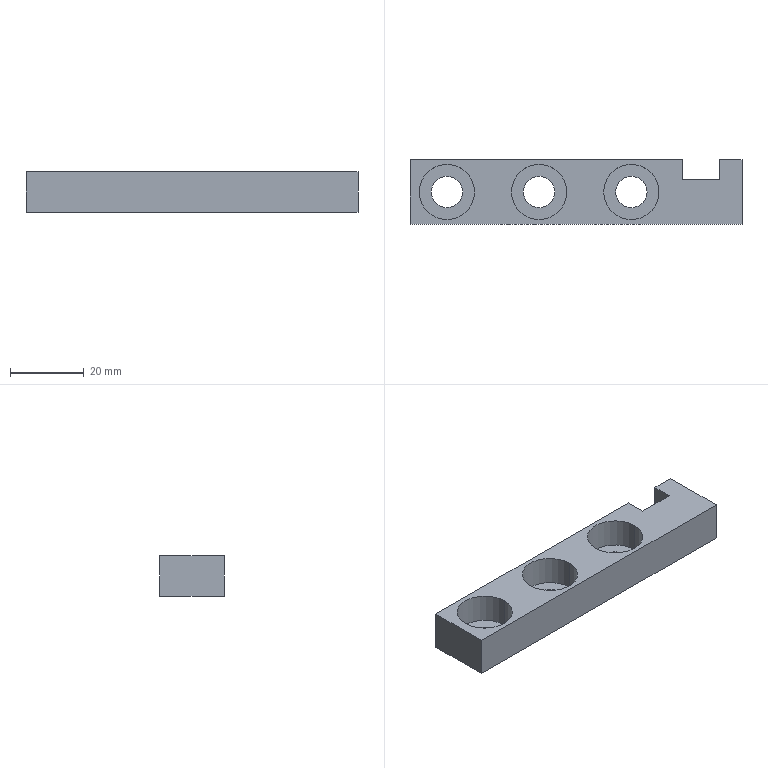Part | SolidWorks | features Extrusion 1, ICE 1 | 1 solid | 25 faces | box 90 x 17.5 x 11 mm | volume 11956 mm3 | plane 13 | cylinder 12 | commonest cylinder face diameters 8.5 x6 15 x6
STEP:
#1=CARTESIAN_POINT('',(-17.5,0.,3.));
#2=VERTEX_POINT('',#1);
#3=CARTESIAN_POINT('',(-2.5,0.,3.));
#4=VERTEX_POINT('',#3);
#5=CARTESIAN_POINT('',(-10.,0.,3.));
#6=DIRECTION('',(0.,0.,1.));
#7=DIRECTION('',(1.,0.,0.));
#8=AXIS2_PLACEMENT_3D('',#5,#6,#7);
#9=CIRCLE('',#8,7.5);
#10=EDGE_CURVE('',#2,#4,#9,.T.);
#11=ORIENTED_EDGE('',*,*,#10,.F.);
#12=CARTESIAN_POINT('',(-17.5,0.,11.));
#13=VERTEX_POINT('',#12);
#14=CARTESIAN_POINT('',(-17.5,0.,3.));
#15=DIRECTION('',(0.,0.,1.));
#16=VECTOR('',#15,1000.);
#17=LINE('',#14,#16);
#18=EDGE_CURVE('',#2,#13,#17,.T.);
#19=ORIENTED_EDGE('',*,*,#18,.T.);
#20=CARTESIAN_POINT('',(-2.5,0.,11.));
#21=VERTEX_POINT('',#20);
#22=CARTESIAN_POINT('',(-10.,0.,11.));
#23=DIRECTION('',(0.,0.,1.));
#24=DIRECTION('',(1.,0.,0.));
#25=AXIS2_PLACEMENT_3D('',#22,#23,#24);
#26=CIRCLE('',#25,7.5);
#27=EDGE_CURVE('',#13,#21,#26,.T.);
#28=ORIENTED_EDGE('',*,*,#27,.T.);
#29=CARTESIAN_POINT('',(-2.5,0.,3.));
#30=DIRECTION('',(0.,0.,1.));
#31=VECTOR('',#30,1000.);
#32=LINE('',#29,#31);
#33=EDGE_CURVE('',#4,#21,#32,.T.);
#34=ORIENTED_EDGE('',*,*,#33,.F.);
#35=EDGE_LOOP('',(#11,#19,#28,#34));
#36=FACE_OUTER_BOUND('',#35,.T.);
#37=CARTESIAN_POINT('',(-10.,0.,3.));
#38=DIRECTION('',(0.,0.,1.));
#39=DIRECTION('',(1.,0.,0.));
#40=AXIS2_PLACEMENT_3D('',#37,#38,#39);
#41=CYLINDRICAL_SURFACE('',#40,7.5);
#42=ADVANCED_FACE('',(#36),#41,.F.);
#43=CARTESIAN_POINT('',(7.5,0.,3.));
#44=VERTEX_POINT('',#43);
#45=CARTESIAN_POINT('',(22.5,0.,3.));
#46=VERTEX_POINT('',#45);
#47=CARTESIAN_POINT('',(15.,0.,3.));
#48=DIRECTION('',(0.,0.,1.));
#49=DIRECTION('',(1.,0.,0.));
#50=AXIS2_PLACEMENT_3D('',#47,#48,#49);
#51=CIRCLE('',#50,7.5);
#52=EDGE_CURVE('',#44,#46,#51,.T.);
#53=ORIENTED_EDGE('',*,*,#52,.F.);
#54=CARTESIAN_POINT('',(7.5,0.,11.));
#55=VERTEX_POINT('',#54);
#56=CARTESIAN_POINT('',(7.5,0.,3.));
#57=DIRECTION('',(0.,0.,1.));
#58=VECTOR('',#57,1000.);
#59=LINE('',#56,#58);
#60=EDGE_CURVE('',#44,#55,#59,.T.);
#61=ORIENTED_EDGE('',*,*,#60,.T.);
#62=CARTESIAN_POINT('',(22.5,0.,11.));
#63=VERTEX_POINT('',#62);
#64=CARTESIAN_POINT('',(15.,0.,11.));
#65=DIRECTION('',(0.,0.,1.));
#66=DIRECTION('',(1.,0.,0.));
#67=AXIS2_PLACEMENT_3D('',#64,#65,#66);
#68=CIRCLE('',#67,7.5);
#69=EDGE_CURVE('',#55,#63,#68,.T.);
#70=ORIENTED_EDGE('',*,*,#69,.T.);
#71=CARTESIAN_POINT('',(22.5,0.,3.));
#72=DIRECTION('',(0.,0.,1.));
#73=VECTOR('',#72,1000.);
#74=LINE('',#71,#73);
#75=EDGE_CURVE('',#46,#63,#74,.T.);
#76=ORIENTED_EDGE('',*,*,#75,.F.);
#77=EDGE_LOOP('',(#53,#61,#70,#76));
#78=FACE_OUTER_BOUND('',#77,.T.);
#79=CARTESIAN_POINT('',(15.,0.,3.));
#80=DIRECTION('',(0.,0.,1.));
#81=DIRECTION('',(1.,0.,0.));
#82=AXIS2_PLACEMENT_3D('',#79,#80,#81);
#83=CYLINDRICAL_SURFACE('',#82,7.5);
#84=ADVANCED_FACE('',(#78),#83,.F.);
#85=CARTESIAN_POINT('',(-42.5,0.,3.));
#86=VERTEX_POINT('',#85);
#87=CARTESIAN_POINT('',(-27.5,0.,3.));
#88=VERTEX_POINT('',#87);
#89=CARTESIAN_POINT('',(-35.,0.,3.));
#90=DIRECTION('',(0.,0.,1.));
#91=DIRECTION('',(1.,0.,0.));
#92=AXIS2_PLACEMENT_3D('',#89,#90,#91);
#93=CIRCLE('',#92,7.5);
#94=EDGE_CURVE('',#86,#88,#93,.T.);
#95=ORIENTED_EDGE('',*,*,#94,.F.);
#96=CARTESIAN_POINT('',(-42.5,0.,11.));
#97=VERTEX_POINT('',#96);
#98=CARTESIAN_POINT('',(-42.5,0.,3.));
#99=DIRECTION('',(0.,0.,1.));
#100=VECTOR('',#99,1000.);
#101=LINE('',#98,#100);
#102=EDGE_CURVE('',#86,#97,#101,.T.);
#103=ORIENTED_EDGE('',*,*,#102,.T.);
#104=CARTESIAN_POINT('',(-27.5,0.,11.));
#105=VERTEX_POINT('',#104);
#106=CARTESIAN_POINT('',(-35.,0.,11.));
#107=DIRECTION('',(0.,0.,1.));
#108=DIRECTION('',(1.,0.,0.));
#109=AXIS2_PLACEMENT_3D('',#106,#107,#108);
#110=CIRCLE('',#109,7.5);
#111=EDGE_CURVE('',#97,#105,#110,.T.);
#112=ORIENTED_EDGE('',*,*,#111,.T.);
#113=CARTESIAN_POINT('',(-27.5,0.,3.));
#114=DIRECTION('',(0.,0.,1.));
#115=VECTOR('',#114,1000.);
#116=LINE('',#113,#115);
#117=EDGE_CURVE('',#88,#105,#116,.T.);
#118=ORIENTED_EDGE('',*,*,#117,.F.);
#119=EDGE_LOOP('',(#95,#103,#112,#118));
#120=FACE_OUTER_BOUND('',#119,.T.);
#121=CARTESIAN_POINT('',(-35.,0.,3.));
#122=DIRECTION('',(0.,0.,1.));
#123=DIRECTION('',(1.,0.,0.));
#124=AXIS2_PLACEMENT_3D('',#121,#122,#123);
#125=CYLINDRICAL_SURFACE('',#124,7.5);
#126=ADVANCED_FACE('',(#120),#125,.F.);
#127=CARTESIAN_POINT('',(-39.25,0.,3.));
#128=VERTEX_POINT('',#127);
#129=CARTESIAN_POINT('',(-30.75,0.,3.));
#130=VERTEX_POINT('',#129);
#131=CARTESIAN_POINT('',(-35.,0.,3.));
#132=DIRECTION('',(0.,0.,1.));
#133=DIRECTION('',(1.,0.,0.));
#134=AXIS2_PLACEMENT_3D('',#131,#132,#133);
#135=CIRCLE('',#134,4.25);
#136=EDGE_CURVE('',#128,#130,#135,.T.);
#137=ORIENTED_EDGE('',*,*,#136,.T.);
#138=CARTESIAN_POINT('',(-30.75,0.,0.));
#139=VERTEX_POINT('',#138);
#140=CARTESIAN_POINT('',(-30.75,0.,11.));
#141=DIRECTION('',(0.,0.,-1.));
#142=VECTOR('',#141,1000.);
#143=LINE('',#140,#142);
#144=EDGE_CURVE('',#130,#139,#143,.T.);
#145=ORIENTED_EDGE('',*,*,#144,.T.);
#146=CARTESIAN_POINT('',(-39.25,0.,0.));
#147=VERTEX_POINT('',#146);
#148=CARTESIAN_POINT('',(-35.,0.,0.));
#149=DIRECTION('',(0.,0.,1.));
#150=DIRECTION('',(1.,0.,0.));
#151=AXIS2_PLACEMENT_3D('',#148,#149,#150);
#152=CIRCLE('',#151,4.25);
#153=EDGE_CURVE('',#147,#139,#152,.T.);
#154=ORIENTED_EDGE('',*,*,#153,.F.);
#155=CARTESIAN_POINT('',(-39.25,0.,11.));
#156=DIRECTION('',(0.,0.,-1.));
#157=VECTOR('',#156,1000.);
#158=LINE('',#155,#157);
#159=EDGE_CURVE('',#128,#147,#158,.T.);
#160=ORIENTED_EDGE('',*,*,#159,.F.);
#161=EDGE_LOOP('',(#137,#145,#154,#160));
#162=FACE_OUTER_BOUND('',#161,.T.);
#163=CARTESIAN_POINT('',(-35.,0.,11.));
#164=DIRECTION('',(0.,0.,-1.));
#165=DIRECTION('',(-1.,0.,0.));
#166=AXIS2_PLACEMENT_3D('',#163,#164,#165);
#167=CYLINDRICAL_SURFACE('',#166,4.25);
#168=ADVANCED_FACE('',(#162),#167,.F.);
#169=CARTESIAN_POINT('',(10.75,0.,3.));
#170=VERTEX_POINT('',#169);
#171=CARTESIAN_POINT('',(19.25,0.,3.));
#172=VERTEX_POINT('',#171);
#173=CARTESIAN_POINT('',(15.,0.,3.));
#174=DIRECTION('',(0.,0.,1.));
#175=DIRECTION('',(1.,0.,0.));
#176=AXIS2_PLACEMENT_3D('',#173,#174,#175);
#177=CIRCLE('',#176,4.25);
#178=EDGE_CURVE('',#170,#172,#177,.T.);
#179=ORIENTED_EDGE('',*,*,#178,.T.);
#180=CARTESIAN_POINT('',(19.25,0.,0.));
#181=VERTEX_POINT('',#180);
#182=CARTESIAN_POINT('',(19.25,0.,11.));
#183=DIRECTION('',(0.,0.,-1.));
#184=VECTOR('',#183,1000.);
#185=LINE('',#182,#184);
#186=EDGE_CURVE('',#172,#181,#185,.T.);
#187=ORIENTED_EDGE('',*,*,#186,.T.);
#188=CARTESIAN_POINT('',(10.75,0.,0.));
#189=VERTEX_POINT('',#188);
#190=CARTESIAN_POINT('',(15.,0.,0.));
#191=DIRECTION('',(0.,0.,1.));
#192=DIRECTION('',(1.,0.,0.));
#193=AXIS2_PLACEMENT_3D('',#190,#191,#192);
#194=CIRCLE('',#193,4.25);
#195=EDGE_CURVE('',#189,#181,#194,.T.);
#196=ORIENTED_EDGE('',*,*,#195,.F.);
#197=CARTESIAN_POINT('',(10.75,0.,11.));
#198=DIRECTION('',(0.,0.,-1.));
#199=VECTOR('',#198,1000.);
#200=LINE('',#197,#199);
#201=EDGE_CURVE('',#170,#189,#200,.T.);
#202=ORIENTED_EDGE('',*,*,#201,.F.);
#203=EDGE_LOOP('',(#179,#187,#196,#202));
#204=FACE_OUTER_BOUND('',#203,.T.);
#205=CARTESIAN_POINT('',(15.,0.,11.));
#206=DIRECTION('',(0.,0.,-1.));
#207=DIRECTION('',(-1.,0.,0.));
#208=AXIS2_PLACEMENT_3D('',#205,#206,#207);
#209=CYLINDRICAL_SURFACE('',#208,4.25);
#210=ADVANCED_FACE('',(#204),#209,.F.);
#211=CARTESIAN_POINT('',(-14.25,0.,3.));
#212=VERTEX_POINT('',#211);
#213=CARTESIAN_POINT('',(-5.75,0.,3.));
#214=VERTEX_POINT('',#213);
#215=CARTESIAN_POINT('',(-10.,0.,3.));
#216=DIRECTION('',(0.,0.,1.));
#217=DIRECTION('',(1.,0.,0.));
#218=AXIS2_PLACEMENT_3D('',#215,#216,#217);
#219=CIRCLE('',#218,4.25);
#220=EDGE_CURVE('',#212,#214,#219,.T.);
#221=ORIENTED_EDGE('',*,*,#220,.T.);
#222=CARTESIAN_POINT('',(-5.75,0.,0.));
#223=VERTEX_POINT('',#222);
#224=CARTESIAN_POINT('',(-5.75,0.,11.));
#225=DIRECTION('',(0.,0.,-1.));
#226=VECTOR('',#225,1000.);
#227=LINE('',#224,#226);
#228=EDGE_CURVE('',#214,#223,#227,.T.);
#229=ORIENTED_EDGE('',*,*,#228,.T.);
#230=CARTESIAN_POINT('',(-14.25,0.,0.));
#231=VERTEX_POINT('',#230);
#232=CARTESIAN_POINT('',(-10.,0.,0.));
#233=DIRECTION('',(0.,0.,1.));
#234=DIRECTION('',(1.,0.,0.));
#235=AXIS2_PLACEMENT_3D('',#232,#233,#234);
#236=CIRCLE('',#235,4.25);
#237=EDGE_CURVE('',#231,#223,#236,.T.);
#238=ORIENTED_EDGE('',*,*,#237,.F.);
#239=CARTESIAN_POINT('',(-14.25,0.,11.));
#240=DIRECTION('',(0.,0.,-1.));
#241=VECTOR('',#240,1000.);
#242=LINE('',#239,#241);
#243=EDGE_CURVE('',#212,#231,#242,.T.);
#244=ORIENTED_EDGE('',*,*,#243,.F.);
#245=EDGE_LOOP('',(#221,#229,#238,#244));
#246=FACE_OUTER_BOUND('',#245,.T.);
#247=CARTESIAN_POINT('',(-10.,0.,11.));
#248=DIRECTION('',(0.,0.,-1.));
#249=DIRECTION('',(-1.,0.,0.));
#250=AXIS2_PLACEMENT_3D('',#247,#248,#249);
#251=CYLINDRICAL_SURFACE('',#250,4.25);
#252=ADVANCED_FACE('',(#246),#251,.F.);
#253=ORIENTED_EDGE('',*,*,#228,.F.);
#254=CARTESIAN_POINT('',(-10.,0.,3.));
#255=DIRECTION('',(0.,0.,1.));
#256=DIRECTION('',(1.,0.,0.));
#257=AXIS2_PLACEMENT_3D('',#254,#255,#256);
#258=CIRCLE('',#257,4.25);
#259=EDGE_CURVE('',#214,#212,#258,.T.);
#260=ORIENTED_EDGE('',*,*,#259,.T.);
#261=ORIENTED_EDGE('',*,*,#243,.T.);
#262=CARTESIAN_POINT('',(-10.,0.,0.));
#263=DIRECTION('',(0.,0.,1.));
#264=DIRECTION('',(1.,0.,0.));
#265=AXIS2_PLACEMENT_3D('',#262,#263,#264);
#266=CIRCLE('',#265,4.25);
#267=EDGE_CURVE('',#223,#231,#266,.T.);
#268=ORIENTED_EDGE('',*,*,#267,.F.);
#269=EDGE_LOOP('',(#253,#260,#261,#268));
#270=FACE_OUTER_BOUND('',#269,.T.);
#271=CARTESIAN_POINT('',(-10.,0.,11.));
#272=DIRECTION('',(0.,0.,-1.));
#273=DIRECTION('',(-1.,0.,0.));
#274=AXIS2_PLACEMENT_3D('',#271,#272,#273);
#275=CYLINDRICAL_SURFACE('',#274,4.25);
#276=ADVANCED_FACE('',(#270),#275,.F.);
#277=ORIENTED_EDGE('',*,*,#186,.F.);
#278=CARTESIAN_POINT('',(15.,0.,3.));
#279=DIRECTION('',(0.,0.,1.));
#280=DIRECTION('',(1.,0.,0.));
#281=AXIS2_PLACEMENT_3D('',#278,#279,#280);
#282=CIRCLE('',#281,4.25);
#283=EDGE_CURVE('',#172,#170,#282,.T.);
#284=ORIENTED_EDGE('',*,*,#283,.T.);
#285=ORIENTED_EDGE('',*,*,#201,.T.);
#286=CARTESIAN_POINT('',(15.,0.,0.));
#287=DIRECTION('',(0.,0.,1.));
#288=DIRECTION('',(1.,0.,0.));
#289=AXIS2_PLACEMENT_3D('',#286,#287,#288);
#290=CIRCLE('',#289,4.25);
#291=EDGE_CURVE('',#181,#189,#290,.T.);
#292=ORIENTED_EDGE('',*,*,#291,.F.);
#293=EDGE_LOOP('',(#277,#284,#285,#292));
#294=FACE_OUTER_BOUND('',#293,.T.);
#295=CARTESIAN_POINT('',(15.,0.,11.));
#296=DIRECTION('',(0.,0.,-1.));
#297=DIRECTION('',(-1.,0.,0.));
#298=AXIS2_PLACEMENT_3D('',#295,#296,#297);
#299=CYLINDRICAL_SURFACE('',#298,4.25);
#300=ADVANCED_FACE('',(#294),#299,.F.);
#301=ORIENTED_EDGE('',*,*,#144,.F.);
#302=CARTESIAN_POINT('',(-35.,0.,3.));
#303=DIRECTION('',(0.,0.,1.));
#304=DIRECTION('',(1.,0.,0.));
#305=AXIS2_PLACEMENT_3D('',#302,#303,#304);
#306=CIRCLE('',#305,4.25);
#307=EDGE_CURVE('',#130,#128,#306,.T.);
#308=ORIENTED_EDGE('',*,*,#307,.T.);
#309=ORIENTED_EDGE('',*,*,#159,.T.);
#310=CARTESIAN_POINT('',(-35.,0.,0.));
#311=DIRECTION('',(0.,0.,1.));
#312=DIRECTION('',(1.,0.,0.));
#313=AXIS2_PLACEMENT_3D('',#310,#311,#312);
#314=CIRCLE('',#313,4.25);
#315=EDGE_CURVE('',#139,#147,#314,.T.);
#316=ORIENTED_EDGE('',*,*,#315,.F.);
#317=EDGE_LOOP('',(#301,#308,#309,#316));
#318=FACE_OUTER_BOUND('',#317,.T.);
#319=CARTESIAN_POINT('',(-35.,0.,11.));
#320=DIRECTION('',(0.,0.,-1.));
#321=DIRECTION('',(-1.,0.,0.));
#322=AXIS2_PLACEMENT_3D('',#319,#320,#321);
#323=CYLINDRICAL_SURFACE('',#322,4.25);
#324=ADVANCED_FACE('',(#318),#323,.F.);
#325=CARTESIAN_POINT('',(-10.,0.,11.));
#326=DIRECTION('',(0.,0.,1.));
#327=DIRECTION('',(1.,0.,0.));
#328=AXIS2_PLACEMENT_3D('',#325,#326,#327);
#329=CIRCLE('',#328,7.5);
#330=EDGE_CURVE('',#21,#13,#329,.T.);
#331=ORIENTED_EDGE('',*,*,#330,.F.);
#332=ORIENTED_EDGE('',*,*,#27,.F.);
#333=EDGE_LOOP('',(#331,#332));
#334=FACE_BOUND('',#333,.T.);
#335=CARTESIAN_POINT('',(15.,0.,11.));
#336=DIRECTION('',(0.,0.,1.));
#337=DIRECTION('',(1.,0.,0.));
#338=AXIS2_PLACEMENT_3D('',#335,#336,#337);
#339=CIRCLE('',#338,7.5);
#340=EDGE_CURVE('',#63,#55,#339,.T.);
#341=ORIENTED_EDGE('',*,*,#340,.F.);
#342=ORIENTED_EDGE('',*,*,#69,.F.);
#343=EDGE_LOOP('',(#341,#342));
#344=FACE_BOUND('',#343,.T.);
#345=CARTESIAN_POINT('',(-35.,0.,11.));
#346=DIRECTION('',(0.,0.,1.));
#347=DIRECTION('',(1.,0.,0.));
#348=AXIS2_PLACEMENT_3D('',#345,#346,#347);
#349=CIRCLE('',#348,7.5);
#350=EDGE_CURVE('',#105,#97,#349,.T.);
#351=ORIENTED_EDGE('',*,*,#350,.F.);
#352=ORIENTED_EDGE('',*,*,#111,.F.);
#353=EDGE_LOOP('',(#351,#352));
#354=FACE_BOUND('',#353,.T.);
#355=CARTESIAN_POINT('',(45.,-8.75,11.));
#356=VERTEX_POINT('',#355);
#357=CARTESIAN_POINT('',(45.,8.75,11.));
#358=VERTEX_POINT('',#357);
#359=CARTESIAN_POINT('',(45.,8.75,11.));
#360=DIRECTION('',(0.,1.,0.));
#361=VECTOR('',#360,1000.);
#362=LINE('',#359,#361);
#363=EDGE_CURVE('',#356,#358,#362,.T.);
#364=ORIENTED_EDGE('',*,*,#363,.T.);
#365=CARTESIAN_POINT('',(39.,8.75,11.));
#366=VERTEX_POINT('',#365);
#367=CARTESIAN_POINT('',(39.,8.75,11.));
#368=DIRECTION('',(-1.,0.,0.));
#369=VECTOR('',#368,1000.);
#370=LINE('',#367,#369);
#371=EDGE_CURVE('',#358,#366,#370,.T.);
#372=ORIENTED_EDGE('',*,*,#371,.T.);
#373=CARTESIAN_POINT('',(39.,3.25,11.));
#374=VERTEX_POINT('',#373);
#375=CARTESIAN_POINT('',(39.,3.25,11.));
#376=DIRECTION('',(0.,-1.,0.));
#377=VECTOR('',#376,1000.);
#378=LINE('',#375,#377);
#379=EDGE_CURVE('',#366,#374,#378,.T.);
#380=ORIENTED_EDGE('',*,*,#379,.T.);
#381=CARTESIAN_POINT('',(28.8,3.25,11.));
#382=VERTEX_POINT('',#381);
#383=CARTESIAN_POINT('',(28.8,3.25,11.));
#384=DIRECTION('',(-1.,0.,0.));
#385=VECTOR('',#384,1000.);
#386=LINE('',#383,#385);
#387=EDGE_CURVE('',#374,#382,#386,.T.);
#388=ORIENTED_EDGE('',*,*,#387,.T.);
#389=CARTESIAN_POINT('',(28.8,8.75,11.));
#390=VERTEX_POINT('',#389);
#391=CARTESIAN_POINT('',(28.8,8.75,11.));
#392=DIRECTION('',(0.,1.,0.));
#393=VECTOR('',#392,1000.);
#394=LINE('',#391,#393);
#395=EDGE_CURVE('',#382,#390,#394,.T.);
#396=ORIENTED_EDGE('',*,*,#395,.T.);
#397=CARTESIAN_POINT('',(-45.,8.75,11.));
#398=VERTEX_POINT('',#397);
#399=CARTESIAN_POINT('',(-45.,8.75,11.));
#400=DIRECTION('',(-1.,0.,0.));
#401=VECTOR('',#400,1000.);
#402=LINE('',#399,#401);
#403=EDGE_CURVE('',#390,#398,#402,.T.);
#404=ORIENTED_EDGE('',*,*,#403,.T.);
#405=CARTESIAN_POINT('',(-45.,-8.75,11.));
#406=VERTEX_POINT('',#405);
#407=CARTESIAN_POINT('',(-45.,8.75,11.));
#408=DIRECTION('',(0.,-1.,0.));
#409=VECTOR('',#408,1000.);
#410=LINE('',#407,#409);
#411=EDGE_CURVE('',#398,#406,#410,.T.);
#412=ORIENTED_EDGE('',*,*,#411,.T.);
#413=CARTESIAN_POINT('',(-45.,-8.75,11.));
#414=DIRECTION('',(1.,0.,0.));
#415=VECTOR('',#414,1000.);
#416=LINE('',#413,#415);
#417=EDGE_CURVE('',#406,#356,#416,.T.);
#418=ORIENTED_EDGE('',*,*,#417,.T.);
#419=EDGE_LOOP('',(#364,#372,#380,#388,#396,#404,#412,#418));
#420=FACE_OUTER_BOUND('',#419,.T.);
#421=CARTESIAN_POINT('',(0.,0.,11.));
#422=DIRECTION('',(0.,0.,1.));
#423=DIRECTION('',(1.,0.,0.));
#424=AXIS2_PLACEMENT_3D('',#421,#422,#423);
#425=PLANE('',#424);
#426=ADVANCED_FACE('',(#334,#344,#354,#420),#425,.T.);
#427=CARTESIAN_POINT('',(45.,-8.75,0.));
#428=VERTEX_POINT('',#427);
#429=CARTESIAN_POINT('',(45.,8.75,0.));
#430=VERTEX_POINT('',#429);
#431=CARTESIAN_POINT('',(45.,8.75,0.));
#432=DIRECTION('',(0.,1.,0.));
#433=VECTOR('',#432,1000.);
#434=LINE('',#431,#433);
#435=EDGE_CURVE('',#428,#430,#434,.T.);
#436=ORIENTED_EDGE('',*,*,#435,.F.);
#437=CARTESIAN_POINT('',(-45.,-8.75,0.));
#438=VERTEX_POINT('',#437);
#439=CARTESIAN_POINT('',(-45.,-8.75,0.));
#440=DIRECTION('',(1.,0.,0.));
#441=VECTOR('',#440,1000.);
#442=LINE('',#439,#441);
#443=EDGE_CURVE('',#438,#428,#442,.T.);
#444=ORIENTED_EDGE('',*,*,#443,.F.);
#445=CARTESIAN_POINT('',(-45.,8.75,0.));
#446=VERTEX_POINT('',#445);
#447=CARTESIAN_POINT('',(-45.,8.75,0.));
#448=DIRECTION('',(0.,-1.,0.));
#449=VECTOR('',#448,1000.);
#450=LINE('',#447,#449);
#451=EDGE_CURVE('',#446,#438,#450,.T.);
#452=ORIENTED_EDGE('',*,*,#451,.F.);
#453=CARTESIAN_POINT('',(28.8,8.75,0.));
#454=VERTEX_POINT('',#453);
#455=CARTESIAN_POINT('',(-45.,8.75,0.));
#456=DIRECTION('',(-1.,0.,0.));
#457=VECTOR('',#456,1000.);
#458=LINE('',#455,#457);
#459=EDGE_CURVE('',#454,#446,#458,.T.);
#460=ORIENTED_EDGE('',*,*,#459,.F.);
#461=CARTESIAN_POINT('',(28.8,3.25,0.));
#462=VERTEX_POINT('',#461);
#463=CARTESIAN_POINT('',(28.8,8.75,0.));
#464=DIRECTION('',(0.,1.,0.));
#465=VECTOR('',#464,1000.);
#466=LINE('',#463,#465);
#467=EDGE_CURVE('',#462,#454,#466,.T.);
#468=ORIENTED_EDGE('',*,*,#467,.F.);
#469=CARTESIAN_POINT('',(39.,3.25,0.));
#470=VERTEX_POINT('',#469);
#471=CARTESIAN_POINT('',(28.8,3.25,0.));
#472=DIRECTION('',(-1.,0.,0.));
#473=VECTOR('',#472,1000.);
#474=LINE('',#471,#473);
#475=EDGE_CURVE('',#470,#462,#474,.T.);
#476=ORIENTED_EDGE('',*,*,#475,.F.);
#477=CARTESIAN_POINT('',(39.,8.75,0.));
#478=VERTEX_POINT('',#477);
#479=CARTESIAN_POINT('',(39.,3.25,0.));
#480=DIRECTION('',(0.,-1.,0.));
#481=VECTOR('',#480,1000.);
#482=LINE('',#479,#481);
#483=EDGE_CURVE('',#478,#470,#482,.T.);
#484=ORIENTED_EDGE('',*,*,#483,.F.);
#485=CARTESIAN_POINT('',(39.,8.75,0.));
#486=DIRECTION('',(-1.,0.,0.));
#487=VECTOR('',#486,1000.);
#488=LINE('',#485,#487);
#489=EDGE_CURVE('',#430,#478,#488,.T.);
#490=ORIENTED_EDGE('',*,*,#489,.F.);
#491=EDGE_LOOP('',(#436,#444,#452,#460,#468,#476,#484,#490));
#492=FACE_OUTER_BOUND('',#491,.T.);
#493=ORIENTED_EDGE('',*,*,#153,.T.);
#494=ORIENTED_EDGE('',*,*,#315,.T.);
#495=EDGE_LOOP('',(#493,#494));
#496=FACE_BOUND('',#495,.T.);
#497=ORIENTED_EDGE('',*,*,#237,.T.);
#498=ORIENTED_EDGE('',*,*,#267,.T.);
#499=EDGE_LOOP('',(#497,#498));
#500=FACE_BOUND('',#499,.T.);
#501=ORIENTED_EDGE('',*,*,#195,.T.);
#502=ORIENTED_EDGE('',*,*,#291,.T.);
#503=EDGE_LOOP('',(#501,#502));
#504=FACE_BOUND('',#503,.T.);
#505=CARTESIAN_POINT('',(0.,0.,0.));
#506=DIRECTION('',(0.,0.,1.));
#507=DIRECTION('',(1.,0.,0.));
#508=AXIS2_PLACEMENT_3D('',#505,#506,#507);
#509=PLANE('',#508);
#510=ADVANCED_FACE('',(#492,#496,#500,#504),#509,.F.);
#511=ORIENTED_EDGE('',*,*,#435,.T.);
#512=CARTESIAN_POINT('',(45.,8.75,11.));
#513=DIRECTION('',(0.,0.,-1.));
#514=VECTOR('',#513,1000.);
#515=LINE('',#512,#514);
#516=EDGE_CURVE('',#358,#430,#515,.T.);
#517=ORIENTED_EDGE('',*,*,#516,.F.);
#518=ORIENTED_EDGE('',*,*,#363,.F.);
#519=CARTESIAN_POINT('',(45.,-8.75,11.));
#520=DIRECTION('',(0.,0.,-1.));
#521=VECTOR('',#520,1000.);
#522=LINE('',#519,#521);
#523=EDGE_CURVE('',#356,#428,#522,.T.);
#524=ORIENTED_EDGE('',*,*,#523,.T.);
#525=EDGE_LOOP('',(#511,#517,#518,#524));
#526=FACE_OUTER_BOUND('',#525,.T.);
#527=CARTESIAN_POINT('',(45.,8.75,11.));
#528=DIRECTION('',(-1.,0.,0.));
#529=DIRECTION('',(0.,0.,1.));
#530=AXIS2_PLACEMENT_3D('',#527,#528,#529);
#531=PLANE('',#530);
#532=ADVANCED_FACE('',(#526),#531,.F.);
#533=ORIENTED_EDGE('',*,*,#489,.T.);
#534=CARTESIAN_POINT('',(39.,8.75,11.));
#535=DIRECTION('',(0.,0.,-1.));
#536=VECTOR('',#535,1000.);
#537=LINE('',#534,#536);
#538=EDGE_CURVE('',#366,#478,#537,.T.);
#539=ORIENTED_EDGE('',*,*,#538,.F.);
#540=ORIENTED_EDGE('',*,*,#371,.F.);
#541=ORIENTED_EDGE('',*,*,#516,.T.);
#542=EDGE_LOOP('',(#533,#539,#540,#541));
#543=FACE_OUTER_BOUND('',#542,.T.);
#544=CARTESIAN_POINT('',(39.,8.75,11.));
#545=DIRECTION('',(0.,-1.,0.));
#546=DIRECTION('',(1.,0.,0.));
#547=AXIS2_PLACEMENT_3D('',#544,#545,#546);
#548=PLANE('',#547);
#549=ADVANCED_FACE('',(#543),#548,.F.);
#550=ORIENTED_EDGE('',*,*,#483,.T.);
#551=CARTESIAN_POINT('',(39.,3.25,11.));
#552=DIRECTION('',(0.,0.,-1.));
#553=VECTOR('',#552,1000.);
#554=LINE('',#551,#553);
#555=EDGE_CURVE('',#374,#470,#554,.T.);
#556=ORIENTED_EDGE('',*,*,#555,.F.);
#557=ORIENTED_EDGE('',*,*,#379,.F.);
#558=ORIENTED_EDGE('',*,*,#538,.T.);
#559=EDGE_LOOP('',(#550,#556,#557,#558));
#560=FACE_OUTER_BOUND('',#559,.T.);
#561=CARTESIAN_POINT('',(39.,3.25,11.));
#562=DIRECTION('',(1.,0.,0.));
#563=DIRECTION('',(0.,0.,-1.));
#564=AXIS2_PLACEMENT_3D('',#561,#562,#563);
#565=PLANE('',#564);
#566=ADVANCED_FACE('',(#560),#565,.F.);
#567=ORIENTED_EDGE('',*,*,#475,.T.);
#568=CARTESIAN_POINT('',(28.8,3.25,11.));
#569=DIRECTION('',(0.,0.,-1.));
#570=VECTOR('',#569,1000.);
#571=LINE('',#568,#570);
#572=EDGE_CURVE('',#382,#462,#571,.T.);
#573=ORIENTED_EDGE('',*,*,#572,.F.);
#574=ORIENTED_EDGE('',*,*,#387,.F.);
#575=ORIENTED_EDGE('',*,*,#555,.T.);
#576=EDGE_LOOP('',(#567,#573,#574,#575));
#577=FACE_OUTER_BOUND('',#576,.T.);
#578=CARTESIAN_POINT('',(28.8,3.25,11.));
#579=DIRECTION('',(0.,-1.,0.));
#580=DIRECTION('',(0.,0.,-1.));
#581=AXIS2_PLACEMENT_3D('',#578,#579,#580);
#582=PLANE('',#581);
#583=ADVANCED_FACE('',(#577),#582,.F.);
#584=ORIENTED_EDGE('',*,*,#467,.T.);
#585=CARTESIAN_POINT('',(28.8,8.75,11.));
#586=DIRECTION('',(0.,0.,-1.));
#587=VECTOR('',#586,1000.);
#588=LINE('',#585,#587);
#589=EDGE_CURVE('',#390,#454,#588,.T.);
#590=ORIENTED_EDGE('',*,*,#589,.F.);
#591=ORIENTED_EDGE('',*,*,#395,.F.);
#592=ORIENTED_EDGE('',*,*,#572,.T.);
#593=EDGE_LOOP('',(#584,#590,#591,#592));
#594=FACE_OUTER_BOUND('',#593,.T.);
#595=CARTESIAN_POINT('',(28.8,8.75,11.));
#596=DIRECTION('',(-1.,0.,0.));
#597=DIRECTION('',(0.,0.,1.));
#598=AXIS2_PLACEMENT_3D('',#595,#596,#597);
#599=PLANE('',#598);
#600=ADVANCED_FACE('',(#594),#599,.F.);
#601=ORIENTED_EDGE('',*,*,#459,.T.);
#602=CARTESIAN_POINT('',(-45.,8.75,11.));
#603=DIRECTION('',(0.,0.,-1.));
#604=VECTOR('',#603,1000.);
#605=LINE('',#602,#604);
#606=EDGE_CURVE('',#398,#446,#605,.T.);
#607=ORIENTED_EDGE('',*,*,#606,.F.);
#608=ORIENTED_EDGE('',*,*,#403,.F.);
#609=ORIENTED_EDGE('',*,*,#589,.T.);
#610=EDGE_LOOP('',(#601,#607,#608,#609));
#611=FACE_OUTER_BOUND('',#610,.T.);
#612=CARTESIAN_POINT('',(-45.,8.75,11.));
#613=DIRECTION('',(0.,-1.,0.));
#614=DIRECTION('',(1.,0.,0.));
#615=AXIS2_PLACEMENT_3D('',#612,#613,#614);
#616=PLANE('',#615);
#617=ADVANCED_FACE('',(#611),#616,.F.);
#618=ORIENTED_EDGE('',*,*,#451,.T.);
#619=CARTESIAN_POINT('',(-45.,-8.75,11.));
#620=DIRECTION('',(0.,0.,-1.));
#621=VECTOR('',#620,1000.);
#622=LINE('',#619,#621);
#623=EDGE_CURVE('',#406,#438,#622,.T.);
#624=ORIENTED_EDGE('',*,*,#623,.F.);
#625=ORIENTED_EDGE('',*,*,#411,.F.);
#626=ORIENTED_EDGE('',*,*,#606,.T.);
#627=EDGE_LOOP('',(#618,#624,#625,#626));
#628=FACE_OUTER_BOUND('',#627,.T.);
#629=CARTESIAN_POINT('',(-45.,8.75,11.));
#630=DIRECTION('',(1.,0.,0.));
#631=DIRECTION('',(0.,0.,-1.));
#632=AXIS2_PLACEMENT_3D('',#629,#630,#631);
#633=PLANE('',#632);
#634=ADVANCED_FACE('',(#628),#633,.F.);
#635=ORIENTED_EDGE('',*,*,#443,.T.);
#636=ORIENTED_EDGE('',*,*,#523,.F.);
#637=ORIENTED_EDGE('',*,*,#417,.F.);
#638=ORIENTED_EDGE('',*,*,#623,.T.);
#639=EDGE_LOOP('',(#635,#636,#637,#638));
#640=FACE_OUTER_BOUND('',#639,.T.);
#641=CARTESIAN_POINT('',(-45.,-8.75,11.));
#642=DIRECTION('',(0.,1.,0.));
#643=DIRECTION('',(0.,0.,1.));
#644=AXIS2_PLACEMENT_3D('',#641,#642,#643);
#645=PLANE('',#644);
#646=ADVANCED_FACE('',(#640),#645,.F.);
#647=ORIENTED_EDGE('',*,*,#102,.F.);
#648=CARTESIAN_POINT('',(-35.,0.,3.));
#649=DIRECTION('',(0.,0.,1.));
#650=DIRECTION('',(1.,0.,0.));
#651=AXIS2_PLACEMENT_3D('',#648,#649,#650);
#652=CIRCLE('',#651,7.5);
#653=EDGE_CURVE('',#88,#86,#652,.T.);
#654=ORIENTED_EDGE('',*,*,#653,.F.);
#655=ORIENTED_EDGE('',*,*,#117,.T.);
#656=ORIENTED_EDGE('',*,*,#350,.T.);
#657=EDGE_LOOP('',(#647,#654,#655,#656));
#658=FACE_OUTER_BOUND('',#657,.T.);
#659=CARTESIAN_POINT('',(-35.,0.,3.));
#660=DIRECTION('',(0.,0.,1.));
#661=DIRECTION('',(1.,0.,0.));
#662=AXIS2_PLACEMENT_3D('',#659,#660,#661);
#663=CYLINDRICAL_SURFACE('',#662,7.5);
#664=ADVANCED_FACE('',(#658),#663,.F.);
#665=ORIENTED_EDGE('',*,*,#136,.F.);
#666=ORIENTED_EDGE('',*,*,#307,.F.);
#667=EDGE_LOOP('',(#665,#666));
#668=FACE_BOUND('',#667,.T.);
#669=ORIENTED_EDGE('',*,*,#653,.T.);
#670=ORIENTED_EDGE('',*,*,#94,.T.);
#671=EDGE_LOOP('',(#669,#670));
#672=FACE_OUTER_BOUND('',#671,.T.);
#673=CARTESIAN_POINT('',(-35.,0.,3.));
#674=DIRECTION('',(0.,0.,1.));
#675=DIRECTION('',(1.,0.,0.));
#676=AXIS2_PLACEMENT_3D('',#673,#674,#675);
#677=PLANE('',#676);
#678=ADVANCED_FACE('',(#668,#672),#677,.T.);
#679=ORIENTED_EDGE('',*,*,#60,.F.);
#680=CARTESIAN_POINT('',(15.,0.,3.));
#681=DIRECTION('',(0.,0.,1.));
#682=DIRECTION('',(1.,0.,0.));
#683=AXIS2_PLACEMENT_3D('',#680,#681,#682);
#684=CIRCLE('',#683,7.5);
#685=EDGE_CURVE('',#46,#44,#684,.T.);
#686=ORIENTED_EDGE('',*,*,#685,.F.);
#687=ORIENTED_EDGE('',*,*,#75,.T.);
#688=ORIENTED_EDGE('',*,*,#340,.T.);
#689=EDGE_LOOP('',(#679,#686,#687,#688));
#690=FACE_OUTER_BOUND('',#689,.T.);
#691=CARTESIAN_POINT('',(15.,0.,3.));
#692=DIRECTION('',(0.,0.,1.));
#693=DIRECTION('',(1.,0.,0.));
#694=AXIS2_PLACEMENT_3D('',#691,#692,#693);
#695=CYLINDRICAL_SURFACE('',#694,7.5);
#696=ADVANCED_FACE('',(#690),#695,.F.);
#697=ORIENTED_EDGE('',*,*,#178,.F.);
#698=ORIENTED_EDGE('',*,*,#283,.F.);
#699=EDGE_LOOP('',(#697,#698));
#700=FACE_BOUND('',#699,.T.);
#701=ORIENTED_EDGE('',*,*,#685,.T.);
#702=ORIENTED_EDGE('',*,*,#52,.T.);
#703=EDGE_LOOP('',(#701,#702));
#704=FACE_OUTER_BOUND('',#703,.T.);
#705=CARTESIAN_POINT('',(15.,0.,3.));
#706=DIRECTION('',(0.,0.,1.));
#707=DIRECTION('',(1.,0.,0.));
#708=AXIS2_PLACEMENT_3D('',#705,#706,#707);
#709=PLANE('',#708);
#710=ADVANCED_FACE('',(#700,#704),#709,.T.);
#711=ORIENTED_EDGE('',*,*,#18,.F.);
#712=CARTESIAN_POINT('',(-10.,0.,3.));
#713=DIRECTION('',(0.,0.,1.));
#714=DIRECTION('',(1.,0.,0.));
#715=AXIS2_PLACEMENT_3D('',#712,#713,#714);
#716=CIRCLE('',#715,7.5);
#717=EDGE_CURVE('',#4,#2,#716,.T.);
#718=ORIENTED_EDGE('',*,*,#717,.F.);
#719=ORIENTED_EDGE('',*,*,#33,.T.);
#720=ORIENTED_EDGE('',*,*,#330,.T.);
#721=EDGE_LOOP('',(#711,#718,#719,#720));
#722=FACE_OUTER_BOUND('',#721,.T.);
#723=CARTESIAN_POINT('',(-10.,0.,3.));
#724=DIRECTION('',(0.,0.,1.));
#725=DIRECTION('',(1.,0.,0.));
#726=AXIS2_PLACEMENT_3D('',#723,#724,#725);
#727=CYLINDRICAL_SURFACE('',#726,7.5);
#728=ADVANCED_FACE('',(#722),#727,.F.);
#729=ORIENTED_EDGE('',*,*,#220,.F.);
#730=ORIENTED_EDGE('',*,*,#259,.F.);
#731=EDGE_LOOP('',(#729,#730));
#732=FACE_BOUND('',#731,.T.);
#733=ORIENTED_EDGE('',*,*,#717,.T.);
#734=ORIENTED_EDGE('',*,*,#10,.T.);
#735=EDGE_LOOP('',(#733,#734));
#736=FACE_OUTER_BOUND('',#735,.T.);
#737=CARTESIAN_POINT('',(-10.,0.,3.));
#738=DIRECTION('',(0.,0.,1.));
#739=DIRECTION('',(1.,0.,0.));
#740=AXIS2_PLACEMENT_3D('',#737,#738,#739);
#741=PLANE('',#740);
#742=ADVANCED_FACE('',(#732,#736),#741,.T.);
#743=CLOSED_SHELL('',(#42,#84,#126,#168,#210,#252,#276,#300,#324,#426,#510,#532,#549,#566,#583,#600,#617,#634,#646,#664,#678,#696,#710,#728,#742));
#744=MANIFOLD_SOLID_BREP('',#743);
#745=CARTESIAN_POINT('',(0.,0.,0.));
#746=DIRECTION('',(0.,0.,1.));
#747=DIRECTION('',(1.,0.,0.));
#748=AXIS2_PLACEMENT_3D('',#745,#746,#747);
#749=(LENGTH_UNIT()NAMED_UNIT(*)SI_UNIT(.MILLI.,.METRE.));
#750=UNCERTAINTY_MEASURE_WITH_UNIT(LENGTH_MEASURE(0.00001),#749,'','');
#751=(NAMED_UNIT(*)PLANE_ANGLE_UNIT()SI_UNIT($,.RADIAN.));
#752=(NAMED_UNIT(*)SI_UNIT($,.STERADIAN.)SOLID_ANGLE_UNIT());
#753=(GEOMETRIC_REPRESENTATION_CONTEXT(3)GLOBAL_UNCERTAINTY_ASSIGNED_CONTEXT((#750))GLOBAL_UNIT_ASSIGNED_CONTEXT((#749,#751,#752))REPRESENTATION_CONTEXT('',''));
#754=ADVANCED_BREP_SHAPE_REPRESENTATION('',(#744,#748),#753);